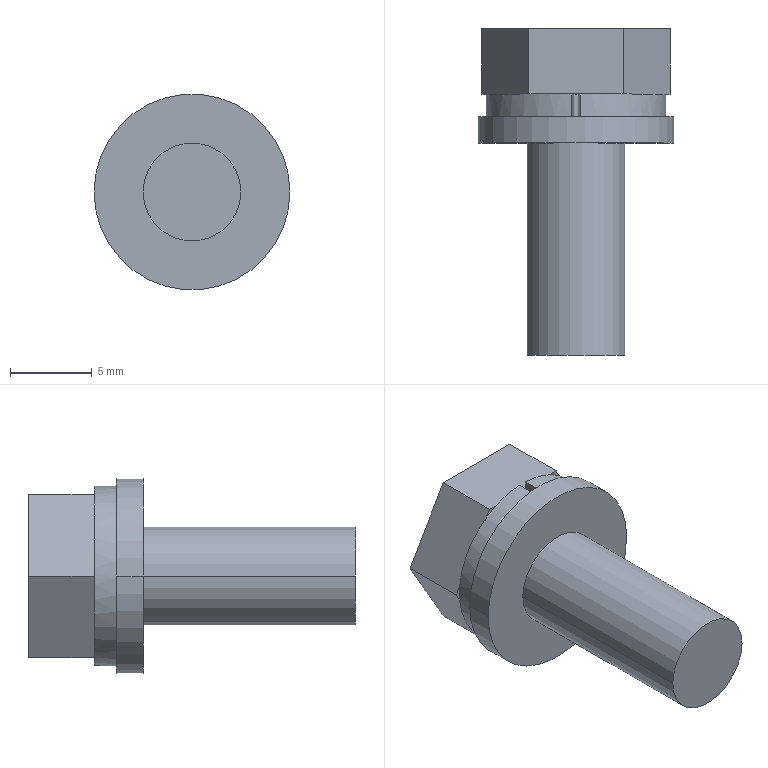Part | STEP file | LIB_36623110_M6X16 | 1 solid | 45 faces | box 12 x 20 x 12 mm | volume 992.686 mm3 | plane 27 | cylinder 18 | commonest cylinder face diameters 0.809 x6 2 x6 6 x3 12 x2 11 x1